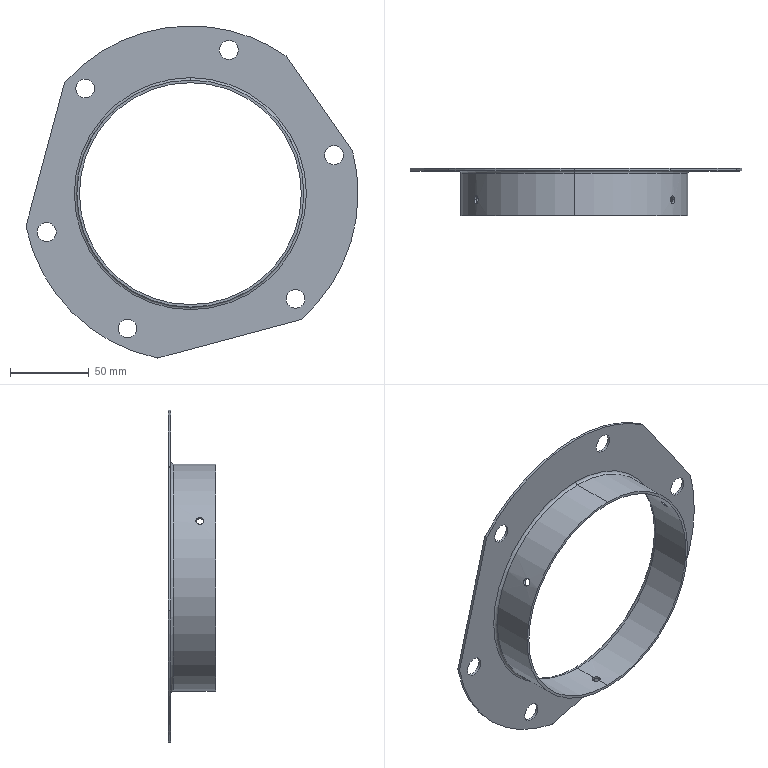Part | SolidWorks | features ICE 3, CirPattern 1, Fillet 1, Revolution 1 | 1 solid | 42 faces | box 210.92 x 30 x 210.92 mm | volume 47725 mm3 | cylinder 32 | plane 6 | torus 4 | commonest cylinder face diameters 12 x12 2 x6 5 x6 213 x4 141 x2 144.2 x2